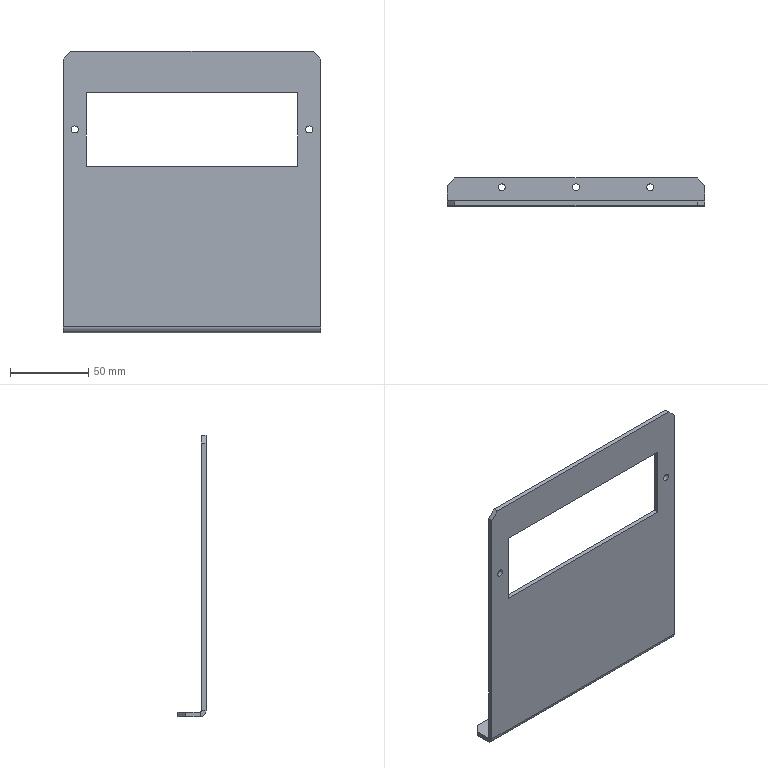Part | NX | 1 solid | 27 faces | box 165 x 18 x 180 mm | volume 76623 mm3 | plane 20 | cylinder 7 | commonest cylinder face diameters 4.5 x5 1.5 x1 7.5 x1
STEP:
#1=CARTESIAN_POINT('',(82.5,0.,3.75));
#2=VERTEX_POINT('',#1);
#3=CARTESIAN_POINT('',(82.5,3.,3.75));
#4=VERTEX_POINT('',#3);
#5=CARTESIAN_POINT('',(82.5,0.,3.75));
#6=DIRECTION('',(0.,1.,0.));
#7=VECTOR('',#6,1000.);
#8=LINE('',#5,#7);
#9=EDGE_CURVE('',#2,#4,#8,.T.);
#10=ORIENTED_EDGE('',*,*,#9,.F.);
#11=CARTESIAN_POINT('',(82.5,3.75,0.));
#12=VERTEX_POINT('',#11);
#13=CARTESIAN_POINT('',(82.5,3.75,3.75));
#14=DIRECTION('',(1.,0.,0.));
#15=DIRECTION('',(0.,0.,-1.));
#16=AXIS2_PLACEMENT_3D('',#13,#14,#15);
#17=CIRCLE('',#16,3.75);
#18=EDGE_CURVE('',#12,#2,#17,.F.);
#19=ORIENTED_EDGE('',*,*,#18,.F.);
#20=CARTESIAN_POINT('',(82.5,3.75,3.));
#21=VERTEX_POINT('',#20);
#22=CARTESIAN_POINT('',(82.5,3.75,3.));
#23=DIRECTION('',(0.,0.,-1.));
#24=VECTOR('',#23,1000.);
#25=LINE('',#22,#24);
#26=EDGE_CURVE('',#21,#12,#25,.T.);
#27=ORIENTED_EDGE('',*,*,#26,.F.);
#28=CARTESIAN_POINT('',(82.5,3.75,3.75));
#29=DIRECTION('',(1.,0.,0.));
#30=DIRECTION('',(0.,0.,-1.));
#31=AXIS2_PLACEMENT_3D('',#28,#29,#30);
#32=CIRCLE('',#31,0.75);
#33=EDGE_CURVE('',#21,#4,#32,.F.);
#34=ORIENTED_EDGE('',*,*,#33,.T.);
#35=EDGE_LOOP('',(#10,#19,#27,#34));
#36=FACE_BOUND('',#35,.T.);
#37=CARTESIAN_POINT('',(82.5,0.,3.75));
#38=DIRECTION('',(1.,0.,0.));
#39=DIRECTION('',(0.,0.,-1.));
#40=AXIS2_PLACEMENT_3D('',#37,#38,#39);
#41=PLANE('',#40);
#42=ADVANCED_FACE('',(#36),#41,.T.);
#43=CARTESIAN_POINT('',(82.5,3.,175.));
#44=VERTEX_POINT('',#43);
#45=CARTESIAN_POINT('',(82.5,3.,0.));
#46=DIRECTION('',(0.,0.,1.));
#47=VECTOR('',#46,1000.);
#48=LINE('',#45,#47);
#49=EDGE_CURVE('',#4,#44,#48,.T.);
#50=ORIENTED_EDGE('',*,*,#49,.T.);
#51=CARTESIAN_POINT('',(82.5,0.,175.));
#52=VERTEX_POINT('',#51);
#53=CARTESIAN_POINT('',(82.5,3.75,175.));
#54=DIRECTION('',(0.,-1.,0.));
#55=VECTOR('',#54,1000.);
#56=LINE('',#53,#55);
#57=EDGE_CURVE('',#44,#52,#56,.T.);
#58=ORIENTED_EDGE('',*,*,#57,.T.);
#59=CARTESIAN_POINT('',(82.5,0.,0.));
#60=DIRECTION('',(0.,0.,1.));
#61=VECTOR('',#60,1000.);
#62=LINE('',#59,#61);
#63=EDGE_CURVE('',#2,#52,#62,.T.);
#64=ORIENTED_EDGE('',*,*,#63,.F.);
#65=ORIENTED_EDGE('',*,*,#9,.T.);
#66=EDGE_LOOP('',(#50,#58,#64,#65));
#67=FACE_BOUND('',#66,.T.);
#68=CARTESIAN_POINT('',(82.5,3.75,3.));
#69=DIRECTION('',(1.,0.,0.));
#70=DIRECTION('',(0.,0.,-1.));
#71=AXIS2_PLACEMENT_3D('',#68,#69,#70);
#72=PLANE('',#71);
#73=ADVANCED_FACE('',(#67),#72,.T.);
#74=CARTESIAN_POINT('',(-82.5,3.75,0.));
#75=VERTEX_POINT('',#74);
#76=CARTESIAN_POINT('',(-82.5,3.75,3.));
#77=VERTEX_POINT('',#76);
#78=CARTESIAN_POINT('',(-82.5,3.75,0.));
#79=DIRECTION('',(0.,0.,1.));
#80=VECTOR('',#79,1000.);
#81=LINE('',#78,#80);
#82=EDGE_CURVE('',#75,#77,#81,.T.);
#83=ORIENTED_EDGE('',*,*,#82,.F.);
#84=CARTESIAN_POINT('',(-82.5,0.,3.75));
#85=VERTEX_POINT('',#84);
#86=CARTESIAN_POINT('',(-82.5,3.75,3.75));
#87=DIRECTION('',(1.,0.,0.));
#88=DIRECTION('',(0.,0.,-1.));
#89=AXIS2_PLACEMENT_3D('',#86,#87,#88);
#90=CIRCLE('',#89,3.75);
#91=EDGE_CURVE('',#75,#85,#90,.F.);
#92=ORIENTED_EDGE('',*,*,#91,.T.);
#93=CARTESIAN_POINT('',(-82.5,3.,3.75));
#94=VERTEX_POINT('',#93);
#95=CARTESIAN_POINT('',(-82.5,3.,3.75));
#96=DIRECTION('',(0.,-1.,0.));
#97=VECTOR('',#96,1000.);
#98=LINE('',#95,#97);
#99=EDGE_CURVE('',#94,#85,#98,.T.);
#100=ORIENTED_EDGE('',*,*,#99,.F.);
#101=CARTESIAN_POINT('',(-82.5,3.75,3.75));
#102=DIRECTION('',(1.,0.,0.));
#103=DIRECTION('',(0.,0.,-1.));
#104=AXIS2_PLACEMENT_3D('',#101,#102,#103);
#105=CIRCLE('',#104,0.75);
#106=EDGE_CURVE('',#77,#94,#105,.F.);
#107=ORIENTED_EDGE('',*,*,#106,.F.);
#108=EDGE_LOOP('',(#83,#92,#100,#107));
#109=FACE_BOUND('',#108,.T.);
#110=CARTESIAN_POINT('',(-82.5,3.75,0.));
#111=DIRECTION('',(-1.,0.,0.));
#112=DIRECTION('',(0.,0.,1.));
#113=AXIS2_PLACEMENT_3D('',#110,#111,#112);
#114=PLANE('',#113);
#115=ADVANCED_FACE('',(#109),#114,.T.);
#116=CARTESIAN_POINT('',(-82.5,13.,3.));
#117=VERTEX_POINT('',#116);
#118=CARTESIAN_POINT('',(-82.5,18.,3.));
#119=DIRECTION('',(0.,-1.,0.));
#120=VECTOR('',#119,1000.);
#121=LINE('',#118,#120);
#122=EDGE_CURVE('',#117,#77,#121,.T.);
#123=ORIENTED_EDGE('',*,*,#122,.F.);
#124=CARTESIAN_POINT('',(-82.5,13.,0.));
#125=VERTEX_POINT('',#124);
#126=CARTESIAN_POINT('',(-82.5,13.,3.75));
#127=DIRECTION('',(0.,0.,-1.));
#128=VECTOR('',#127,1000.);
#129=LINE('',#126,#128);
#130=EDGE_CURVE('',#117,#125,#129,.T.);
#131=ORIENTED_EDGE('',*,*,#130,.T.);
#132=CARTESIAN_POINT('',(-82.5,18.,0.));
#133=DIRECTION('',(0.,-1.,0.));
#134=VECTOR('',#133,1000.);
#135=LINE('',#132,#134);
#136=EDGE_CURVE('',#125,#75,#135,.T.);
#137=ORIENTED_EDGE('',*,*,#136,.T.);
#138=ORIENTED_EDGE('',*,*,#82,.T.);
#139=EDGE_LOOP('',(#123,#131,#137,#138));
#140=FACE_BOUND('',#139,.T.);
#141=CARTESIAN_POINT('',(-82.5,3.,3.75));
#142=DIRECTION('',(-1.,0.,0.));
#143=DIRECTION('',(0.,0.,1.));
#144=AXIS2_PLACEMENT_3D('',#141,#142,#143);
#145=PLANE('',#144);
#146=ADVANCED_FACE('',(#140),#145,.T.);
#147=CARTESIAN_POINT('',(-67.5,3.,106.5));
#148=VERTEX_POINT('',#147);
#149=CARTESIAN_POINT('',(67.5,3.,106.5));
#150=VERTEX_POINT('',#149);
#151=CARTESIAN_POINT('',(82.5,3.,106.5));
#152=DIRECTION('',(1.,0.,0.));
#153=VECTOR('',#152,1000.);
#154=LINE('',#151,#153);
#155=EDGE_CURVE('',#148,#150,#154,.T.);
#156=ORIENTED_EDGE('',*,*,#155,.T.);
#157=CARTESIAN_POINT('',(67.5,3.,153.5));
#158=VERTEX_POINT('',#157);
#159=CARTESIAN_POINT('',(67.5,3.,0.));
#160=DIRECTION('',(0.,0.,1.));
#161=VECTOR('',#160,1000.);
#162=LINE('',#159,#161);
#163=EDGE_CURVE('',#150,#158,#162,.T.);
#164=ORIENTED_EDGE('',*,*,#163,.T.);
#165=CARTESIAN_POINT('',(-67.5,3.,153.5));
#166=VERTEX_POINT('',#165);
#167=CARTESIAN_POINT('',(82.5,3.,153.5));
#168=DIRECTION('',(-1.,0.,0.));
#169=VECTOR('',#168,1000.);
#170=LINE('',#167,#169);
#171=EDGE_CURVE('',#158,#166,#170,.T.);
#172=ORIENTED_EDGE('',*,*,#171,.T.);
#173=CARTESIAN_POINT('',(-67.5,3.,0.));
#174=DIRECTION('',(0.,0.,-1.));
#175=VECTOR('',#174,1000.);
#176=LINE('',#173,#175);
#177=EDGE_CURVE('',#166,#148,#176,.T.);
#178=ORIENTED_EDGE('',*,*,#177,.T.);
#179=EDGE_LOOP('',(#156,#164,#172,#178));
#180=FACE_BOUND('',#179,.T.);
#181=CARTESIAN_POINT('',(75.,3.,127.75));
#182=VERTEX_POINT('',#181);
#183=CARTESIAN_POINT('',(75.,3.,130.));
#184=DIRECTION('',(0.,-1.,0.));
#185=DIRECTION('',(0.,0.,-1.));
#186=AXIS2_PLACEMENT_3D('',#183,#184,#185);
#187=CIRCLE('',#186,2.25);
#188=EDGE_CURVE('',#182,#182,#187,.T.);
#189=ORIENTED_EDGE('',*,*,#188,.T.);
#190=EDGE_LOOP('',(#189));
#191=FACE_BOUND('',#190,.T.);
#192=CARTESIAN_POINT('',(-75.,3.,127.75));
#193=VERTEX_POINT('',#192);
#194=CARTESIAN_POINT('',(-75.,3.,130.));
#195=DIRECTION('',(0.,-1.,0.));
#196=DIRECTION('',(0.,0.,-1.));
#197=AXIS2_PLACEMENT_3D('',#194,#195,#196);
#198=CIRCLE('',#197,2.25);
#199=EDGE_CURVE('',#193,#193,#198,.T.);
#200=ORIENTED_EDGE('',*,*,#199,.T.);
#201=EDGE_LOOP('',(#200));
#202=FACE_BOUND('',#201,.T.);
#203=CARTESIAN_POINT('',(77.5,3.,180.));
#204=VERTEX_POINT('',#203);
#205=CARTESIAN_POINT('',(-77.5,3.,180.));
#206=VERTEX_POINT('',#205);
#207=CARTESIAN_POINT('',(82.5,3.,180.));
#208=DIRECTION('',(-1.,0.,0.));
#209=VECTOR('',#208,1000.);
#210=LINE('',#207,#209);
#211=EDGE_CURVE('',#204,#206,#210,.T.);
#212=ORIENTED_EDGE('',*,*,#211,.F.);
#213=CARTESIAN_POINT('',(77.5,3.,180.));
#214=DIRECTION('',(-0.7071,0.,0.7071));
#215=VECTOR('',#214,1000.);
#216=LINE('',#213,#215);
#217=EDGE_CURVE('',#204,#44,#216,.F.);
#218=ORIENTED_EDGE('',*,*,#217,.T.);
#219=ORIENTED_EDGE('',*,*,#49,.F.);
#220=CARTESIAN_POINT('',(82.5,3.,3.75));
#221=DIRECTION('',(-1.,0.,0.));
#222=VECTOR('',#221,1000.);
#223=LINE('',#220,#222);
#224=EDGE_CURVE('',#4,#94,#223,.T.);
#225=ORIENTED_EDGE('',*,*,#224,.T.);
#226=CARTESIAN_POINT('',(-82.5,3.,175.));
#227=VERTEX_POINT('',#226);
#228=CARTESIAN_POINT('',(-82.5,3.,0.));
#229=DIRECTION('',(0.,0.,1.));
#230=VECTOR('',#229,1000.);
#231=LINE('',#228,#230);
#232=EDGE_CURVE('',#94,#227,#231,.T.);
#233=ORIENTED_EDGE('',*,*,#232,.T.);
#234=CARTESIAN_POINT('',(-82.5,3.,175.));
#235=DIRECTION('',(0.7071,0.,0.7071));
#236=VECTOR('',#235,1000.);
#237=LINE('',#234,#236);
#238=EDGE_CURVE('',#227,#206,#237,.T.);
#239=ORIENTED_EDGE('',*,*,#238,.T.);
#240=EDGE_LOOP('',(#212,#218,#219,#225,#233,#239));
#241=FACE_BOUND('',#240,.T.);
#242=CARTESIAN_POINT('',(82.5,3.,0.));
#243=DIRECTION('',(0.,-1.,0.));
#244=DIRECTION('',(0.,0.,-1.));
#245=AXIS2_PLACEMENT_3D('',#242,#243,#244);
#246=PLANE('',#245);
#247=ADVANCED_FACE('',(#180,#191,#202,#241),#246,.F.);
#248=CARTESIAN_POINT('',(77.5,0.,180.));
#249=VERTEX_POINT('',#248);
#250=CARTESIAN_POINT('',(-77.5,0.,180.));
#251=VERTEX_POINT('',#250);
#252=CARTESIAN_POINT('',(82.5,0.,180.));
#253=DIRECTION('',(-1.,0.,0.));
#254=VECTOR('',#253,1000.);
#255=LINE('',#252,#254);
#256=EDGE_CURVE('',#249,#251,#255,.T.);
#257=ORIENTED_EDGE('',*,*,#256,.F.);
#258=CARTESIAN_POINT('',(77.5,0.,180.));
#259=DIRECTION('',(0.,1.,0.));
#260=VECTOR('',#259,1000.);
#261=LINE('',#258,#260);
#262=EDGE_CURVE('',#249,#204,#261,.T.);
#263=ORIENTED_EDGE('',*,*,#262,.T.);
#264=ORIENTED_EDGE('',*,*,#211,.T.);
#265=CARTESIAN_POINT('',(-77.5,0.,180.));
#266=DIRECTION('',(0.,-1.,0.));
#267=VECTOR('',#266,1000.);
#268=LINE('',#265,#267);
#269=EDGE_CURVE('',#206,#251,#268,.T.);
#270=ORIENTED_EDGE('',*,*,#269,.T.);
#271=EDGE_LOOP('',(#257,#263,#264,#270));
#272=FACE_BOUND('',#271,.T.);
#273=CARTESIAN_POINT('',(82.5,0.,180.));
#274=DIRECTION('',(0.,0.,1.));
#275=DIRECTION('',(1.,0.,0.));
#276=AXIS2_PLACEMENT_3D('',#273,#274,#275);
#277=PLANE('',#276);
#278=ADVANCED_FACE('',(#272),#277,.T.);
#279=CARTESIAN_POINT('',(67.5,0.,106.5));
#280=VERTEX_POINT('',#279);
#281=CARTESIAN_POINT('',(67.5,0.,153.5));
#282=VERTEX_POINT('',#281);
#283=CARTESIAN_POINT('',(67.5,0.,106.5));
#284=DIRECTION('',(0.,0.,1.));
#285=VECTOR('',#284,1000.);
#286=LINE('',#283,#285);
#287=EDGE_CURVE('',#280,#282,#286,.T.);
#288=ORIENTED_EDGE('',*,*,#287,.F.);
#289=CARTESIAN_POINT('',(-67.5,0.,106.5));
#290=VERTEX_POINT('',#289);
#291=CARTESIAN_POINT('',(-67.5,0.,106.5));
#292=DIRECTION('',(1.,0.,0.));
#293=VECTOR('',#292,1000.);
#294=LINE('',#291,#293);
#295=EDGE_CURVE('',#290,#280,#294,.T.);
#296=ORIENTED_EDGE('',*,*,#295,.F.);
#297=CARTESIAN_POINT('',(-67.5,0.,153.5));
#298=VERTEX_POINT('',#297);
#299=CARTESIAN_POINT('',(-67.5,0.,106.5));
#300=DIRECTION('',(0.,0.,-1.));
#301=VECTOR('',#300,1000.);
#302=LINE('',#299,#301);
#303=EDGE_CURVE('',#298,#290,#302,.T.);
#304=ORIENTED_EDGE('',*,*,#303,.F.);
#305=CARTESIAN_POINT('',(-67.5,0.,153.5));
#306=DIRECTION('',(-1.,0.,0.));
#307=VECTOR('',#306,1000.);
#308=LINE('',#305,#307);
#309=EDGE_CURVE('',#282,#298,#308,.T.);
#310=ORIENTED_EDGE('',*,*,#309,.F.);
#311=EDGE_LOOP('',(#288,#296,#304,#310));
#312=FACE_BOUND('',#311,.T.);
#313=CARTESIAN_POINT('',(75.,0.,127.75));
#314=VERTEX_POINT('',#313);
#315=CARTESIAN_POINT('',(75.,0.,130.));
#316=DIRECTION('',(0.,-1.,0.));
#317=DIRECTION('',(0.,0.,-1.));
#318=AXIS2_PLACEMENT_3D('',#315,#316,#317);
#319=CIRCLE('',#318,2.25);
#320=EDGE_CURVE('',#314,#314,#319,.T.);
#321=ORIENTED_EDGE('',*,*,#320,.F.);
#322=EDGE_LOOP('',(#321));
#323=FACE_BOUND('',#322,.T.);
#324=CARTESIAN_POINT('',(-75.,0.,127.75));
#325=VERTEX_POINT('',#324);
#326=CARTESIAN_POINT('',(-75.,0.,130.));
#327=DIRECTION('',(0.,-1.,0.));
#328=DIRECTION('',(0.,0.,-1.));
#329=AXIS2_PLACEMENT_3D('',#326,#327,#328);
#330=CIRCLE('',#329,2.25);
#331=EDGE_CURVE('',#325,#325,#330,.T.);
#332=ORIENTED_EDGE('',*,*,#331,.F.);
#333=EDGE_LOOP('',(#332));
#334=FACE_BOUND('',#333,.T.);
#335=ORIENTED_EDGE('',*,*,#63,.T.);
#336=CARTESIAN_POINT('',(170.,0.,87.5));
#337=DIRECTION('',(0.7071,0.,-0.7071));
#338=VECTOR('',#337,1000.);
#339=LINE('',#336,#338);
#340=EDGE_CURVE('',#52,#249,#339,.F.);
#341=ORIENTED_EDGE('',*,*,#340,.T.);
#342=ORIENTED_EDGE('',*,*,#256,.T.);
#343=CARTESIAN_POINT('',(-82.5,0.,175.));
#344=VERTEX_POINT('',#343);
#345=CARTESIAN_POINT('',(-87.5,0.,170.));
#346=DIRECTION('',(-0.7071,0.,-0.7071));
#347=VECTOR('',#346,1000.);
#348=LINE('',#345,#347);
#349=EDGE_CURVE('',#251,#344,#348,.T.);
#350=ORIENTED_EDGE('',*,*,#349,.T.);
#351=CARTESIAN_POINT('',(-82.5,0.,0.));
#352=DIRECTION('',(0.,0.,1.));
#353=VECTOR('',#352,1000.);
#354=LINE('',#351,#353);
#355=EDGE_CURVE('',#85,#344,#354,.T.);
#356=ORIENTED_EDGE('',*,*,#355,.F.);
#357=CARTESIAN_POINT('',(82.5,0.,3.75));
#358=DIRECTION('',(-1.,0.,0.));
#359=VECTOR('',#358,1000.);
#360=LINE('',#357,#359);
#361=EDGE_CURVE('',#2,#85,#360,.T.);
#362=ORIENTED_EDGE('',*,*,#361,.F.);
#363=EDGE_LOOP('',(#335,#341,#342,#350,#356,#362));
#364=FACE_BOUND('',#363,.T.);
#365=CARTESIAN_POINT('',(82.5,0.,0.));
#366=DIRECTION('',(0.,-1.,0.));
#367=DIRECTION('',(0.,0.,-1.));
#368=AXIS2_PLACEMENT_3D('',#365,#366,#367);
#369=PLANE('',#368);
#370=ADVANCED_FACE('',(#312,#323,#334,#364),#369,.T.);
#371=ORIENTED_EDGE('',*,*,#91,.F.);
#372=CARTESIAN_POINT('',(82.5,3.75,0.));
#373=DIRECTION('',(-1.,0.,0.));
#374=VECTOR('',#373,1000.);
#375=LINE('',#372,#374);
#376=EDGE_CURVE('',#12,#75,#375,.T.);
#377=ORIENTED_EDGE('',*,*,#376,.F.);
#378=ORIENTED_EDGE('',*,*,#18,.T.);
#379=ORIENTED_EDGE('',*,*,#361,.T.);
#380=EDGE_LOOP('',(#371,#377,#378,#379));
#381=FACE_BOUND('',#380,.T.);
#382=CARTESIAN_POINT('',(82.5,3.75,3.75));
#383=DIRECTION('',(-1.,0.,0.));
#384=DIRECTION('',(0.,0.,1.));
#385=AXIS2_PLACEMENT_3D('',#382,#383,#384);
#386=CYLINDRICAL_SURFACE('',#385,3.75);
#387=ADVANCED_FACE('',(#381),#386,.T.);
#388=CARTESIAN_POINT('',(-45.25,12.,0.));
#389=VERTEX_POINT('',#388);
#390=CARTESIAN_POINT('',(-47.5,12.,0.));
#391=DIRECTION('',(0.,0.,1.));
#392=DIRECTION('',(1.,0.,0.));
#393=AXIS2_PLACEMENT_3D('',#390,#391,#392);
#394=CIRCLE('',#393,2.25);
#395=EDGE_CURVE('',#389,#389,#394,.T.);
#396=ORIENTED_EDGE('',*,*,#395,.T.);
#397=EDGE_LOOP('',(#396));
#398=FACE_BOUND('',#397,.T.);
#399=CARTESIAN_POINT('',(49.75,12.,0.));
#400=VERTEX_POINT('',#399);
#401=CARTESIAN_POINT('',(47.5,12.,0.));
#402=DIRECTION('',(0.,0.,1.));
#403=DIRECTION('',(1.,0.,0.));
#404=AXIS2_PLACEMENT_3D('',#401,#402,#403);
#405=CIRCLE('',#404,2.25);
#406=EDGE_CURVE('',#400,#400,#405,.T.);
#407=ORIENTED_EDGE('',*,*,#406,.T.);
#408=EDGE_LOOP('',(#407));
#409=FACE_BOUND('',#408,.T.);
#410=CARTESIAN_POINT('',(2.25,12.,0.));
#411=VERTEX_POINT('',#410);
#412=CARTESIAN_POINT('',(0.,12.,0.));
#413=DIRECTION('',(0.,0.,1.));
#414=DIRECTION('',(1.,0.,0.));
#415=AXIS2_PLACEMENT_3D('',#412,#413,#414);
#416=CIRCLE('',#415,2.25);
#417=EDGE_CURVE('',#411,#411,#416,.T.);
#418=ORIENTED_EDGE('',*,*,#417,.T.);
#419=EDGE_LOOP('',(#418));
#420=FACE_BOUND('',#419,.T.);
#421=CARTESIAN_POINT('',(77.5,18.,0.));
#422=VERTEX_POINT('',#421);
#423=CARTESIAN_POINT('',(-77.5,18.,0.));
#424=VERTEX_POINT('',#423);
#425=CARTESIAN_POINT('',(82.5,18.,0.));
#426=DIRECTION('',(-1.,0.,0.));
#427=VECTOR('',#426,1000.);
#428=LINE('',#425,#427);
#429=EDGE_CURVE('',#422,#424,#428,.T.);
#430=ORIENTED_EDGE('',*,*,#429,.F.);
#431=CARTESIAN_POINT('',(82.5,13.,0.));
#432=VERTEX_POINT('',#431);
#433=CARTESIAN_POINT('',(80.,15.5,0.));
#434=DIRECTION('',(-0.7071,0.7071,0.));
#435=VECTOR('',#434,1000.);
#436=LINE('',#433,#435);
#437=EDGE_CURVE('',#422,#432,#436,.F.);
#438=ORIENTED_EDGE('',*,*,#437,.T.);
#439=CARTESIAN_POINT('',(82.5,18.,0.));
#440=DIRECTION('',(0.,-1.,0.));
#441=VECTOR('',#440,1000.);
#442=LINE('',#439,#441);
#443=EDGE_CURVE('',#432,#12,#442,.T.);
#444=ORIENTED_EDGE('',*,*,#443,.T.);
#445=ORIENTED_EDGE('',*,*,#376,.T.);
#446=ORIENTED_EDGE('',*,*,#136,.F.);
#447=CARTESIAN_POINT('',(2.5,98.,0.));
#448=DIRECTION('',(-0.7071,-0.7071,0.));
#449=VECTOR('',#448,1000.);
#450=LINE('',#447,#449);
#451=EDGE_CURVE('',#125,#424,#450,.F.);
#452=ORIENTED_EDGE('',*,*,#451,.T.);
#453=EDGE_LOOP('',(#430,#438,#444,#445,#446,#452));
#454=FACE_BOUND('',#453,.T.);
#455=CARTESIAN_POINT('',(82.5,18.,0.));
#456=DIRECTION('',(0.,0.,-1.));
#457=DIRECTION('',(0.,1.,0.));
#458=AXIS2_PLACEMENT_3D('',#455,#456,#457);
#459=PLANE('',#458);
#460=ADVANCED_FACE('',(#398,#409,#420,#454),#459,.T.);
#461=CARTESIAN_POINT('',(77.5,18.,3.));
#462=VERTEX_POINT('',#461);
#463=CARTESIAN_POINT('',(-77.5,18.,3.));
#464=VERTEX_POINT('',#463);
#465=CARTESIAN_POINT('',(82.5,18.,3.));
#466=DIRECTION('',(-1.,0.,0.));
#467=VECTOR('',#466,1000.);
#468=LINE('',#465,#467);
#469=EDGE_CURVE('',#462,#464,#468,.T.);
#470=ORIENTED_EDGE('',*,*,#469,.F.);
#471=CARTESIAN_POINT('',(77.5,18.,3.));
#472=DIRECTION('',(0.,0.,-1.));
#473=VECTOR('',#472,1000.);
#474=LINE('',#471,#473);
#475=EDGE_CURVE('',#462,#422,#474,.T.);
#476=ORIENTED_EDGE('',*,*,#475,.T.);
#477=ORIENTED_EDGE('',*,*,#429,.T.);
#478=CARTESIAN_POINT('',(-77.5,18.,3.));
#479=DIRECTION('',(0.,0.,1.));
#480=VECTOR('',#479,1000.);
#481=LINE('',#478,#480);
#482=EDGE_CURVE('',#424,#464,#481,.T.);
#483=ORIENTED_EDGE('',*,*,#482,.T.);
#484=EDGE_LOOP('',(#470,#476,#477,#483));
#485=FACE_BOUND('',#484,.T.);
#486=CARTESIAN_POINT('',(82.5,18.,3.));
#487=DIRECTION('',(0.,1.,0.));
#488=DIRECTION('',(0.,0.,1.));
#489=AXIS2_PLACEMENT_3D('',#486,#487,#488);
#490=PLANE('',#489);
#491=ADVANCED_FACE('',(#485),#490,.T.);
#492=CARTESIAN_POINT('',(-45.25,12.,3.));
#493=VERTEX_POINT('',#492);
#494=CARTESIAN_POINT('',(-47.5,12.,3.));
#495=DIRECTION('',(0.,0.,1.));
#496=DIRECTION('',(1.,0.,0.));
#497=AXIS2_PLACEMENT_3D('',#494,#495,#496);
#498=CIRCLE('',#497,2.25);
#499=EDGE_CURVE('',#493,#493,#498,.T.);
#500=ORIENTED_EDGE('',*,*,#499,.F.);
#501=EDGE_LOOP('',(#500));
#502=FACE_BOUND('',#501,.T.);
#503=CARTESIAN_POINT('',(49.75,12.,3.));
#504=VERTEX_POINT('',#503);
#505=CARTESIAN_POINT('',(47.5,12.,3.));
#506=DIRECTION('',(0.,0.,1.));
#507=DIRECTION('',(1.,0.,0.));
#508=AXIS2_PLACEMENT_3D('',#505,#506,#507);
#509=CIRCLE('',#508,2.25);
#510=EDGE_CURVE('',#504,#504,#509,.T.);
#511=ORIENTED_EDGE('',*,*,#510,.F.);
#512=EDGE_LOOP('',(#511));
#513=FACE_BOUND('',#512,.T.);
#514=CARTESIAN_POINT('',(2.25,12.,3.));
#515=VERTEX_POINT('',#514);
#516=CARTESIAN_POINT('',(0.,12.,3.));
#517=DIRECTION('',(0.,0.,1.));
#518=DIRECTION('',(1.,0.,0.));
#519=AXIS2_PLACEMENT_3D('',#516,#517,#518);
#520=CIRCLE('',#519,2.25);
#521=EDGE_CURVE('',#515,#515,#520,.T.);
#522=ORIENTED_EDGE('',*,*,#521,.F.);
#523=EDGE_LOOP('',(#522));
#524=FACE_BOUND('',#523,.T.);
#525=CARTESIAN_POINT('',(82.5,13.,3.));
#526=VERTEX_POINT('',#525);
#527=CARTESIAN_POINT('',(82.5,18.,3.));
#528=DIRECTION('',(0.,-1.,0.));
#529=VECTOR('',#528,1000.);
#530=LINE('',#527,#529);
#531=EDGE_CURVE('',#526,#21,#530,.T.);
#532=ORIENTED_EDGE('',*,*,#531,.F.);
#533=CARTESIAN_POINT('',(77.5,18.,3.));
#534=DIRECTION('',(0.7071,-0.7071,0.));
#535=VECTOR('',#534,1000.);
#536=LINE('',#533,#535);
#537=EDGE_CURVE('',#526,#462,#536,.F.);
#538=ORIENTED_EDGE('',*,*,#537,.T.);
#539=ORIENTED_EDGE('',*,*,#469,.T.);
#540=CARTESIAN_POINT('',(-82.5,13.,3.));
#541=DIRECTION('',(0.7071,0.7071,0.));
#542=VECTOR('',#541,1000.);
#543=LINE('',#540,#542);
#544=EDGE_CURVE('',#464,#117,#543,.F.);
#545=ORIENTED_EDGE('',*,*,#544,.T.);
#546=ORIENTED_EDGE('',*,*,#122,.T.);
#547=CARTESIAN_POINT('',(82.5,3.75,3.));
#548=DIRECTION('',(-1.,0.,0.));
#549=VECTOR('',#548,1000.);
#550=LINE('',#547,#549);
#551=EDGE_CURVE('',#21,#77,#550,.T.);
#552=ORIENTED_EDGE('',*,*,#551,.F.);
#553=EDGE_LOOP('',(#532,#538,#539,#545,#546,#552));
#554=FACE_BOUND('',#553,.T.);
#555=CARTESIAN_POINT('',(82.5,18.,3.));
#556=DIRECTION('',(0.,0.,-1.));
#557=DIRECTION('',(0.,1.,0.));
#558=AXIS2_PLACEMENT_3D('',#555,#556,#557);
#559=PLANE('',#558);
#560=ADVANCED_FACE('',(#502,#513,#524,#554),#559,.F.);
#561=ORIENTED_EDGE('',*,*,#106,.T.);
#562=ORIENTED_EDGE('',*,*,#224,.F.);
#563=ORIENTED_EDGE('',*,*,#33,.F.);
#564=ORIENTED_EDGE('',*,*,#551,.T.);
#565=EDGE_LOOP('',(#561,#562,#563,#564));
#566=FACE_BOUND('',#565,.T.);
#567=CARTESIAN_POINT('',(82.5,3.75,3.75));
#568=DIRECTION('',(-1.,0.,0.));
#569=DIRECTION('',(0.,0.,1.));
#570=AXIS2_PLACEMENT_3D('',#567,#568,#569);
#571=CYLINDRICAL_SURFACE('',#570,0.75);
#572=ADVANCED_FACE('',(#566),#571,.F.);
#573=ORIENTED_EDGE('',*,*,#443,.F.);
#574=CARTESIAN_POINT('',(82.5,13.,3.75));
#575=DIRECTION('',(0.,0.,1.));
#576=VECTOR('',#575,1000.);
#577=LINE('',#574,#576);
#578=EDGE_CURVE('',#432,#526,#577,.T.);
#579=ORIENTED_EDGE('',*,*,#578,.T.);
#580=ORIENTED_EDGE('',*,*,#531,.T.);
#581=ORIENTED_EDGE('',*,*,#26,.T.);
#582=EDGE_LOOP('',(#573,#579,#580,#581));
#583=FACE_BOUND('',#582,.T.);
#584=CARTESIAN_POINT('',(82.5,3.75,3.75));
#585=DIRECTION('',(1.,0.,0.));
#586=DIRECTION('',(0.,0.,-1.));
#587=AXIS2_PLACEMENT_3D('',#584,#585,#586);
#588=PLANE('',#587);
#589=ADVANCED_FACE('',(#583),#588,.T.);
#590=ORIENTED_EDGE('',*,*,#355,.T.);
#591=CARTESIAN_POINT('',(-82.5,3.,175.));
#592=DIRECTION('',(0.,1.,0.));
#593=VECTOR('',#592,1000.);
#594=LINE('',#591,#593);
#595=EDGE_CURVE('',#344,#227,#594,.T.);
#596=ORIENTED_EDGE('',*,*,#595,.T.);
#597=ORIENTED_EDGE('',*,*,#232,.F.);
#598=ORIENTED_EDGE('',*,*,#99,.T.);
#599=EDGE_LOOP('',(#590,#596,#597,#598));
#600=FACE_BOUND('',#599,.T.);
#601=CARTESIAN_POINT('',(-82.5,3.75,3.75));
#602=DIRECTION('',(1.,0.,0.));
#603=DIRECTION('',(0.,0.,-1.));
#604=AXIS2_PLACEMENT_3D('',#601,#602,#603);
#605=PLANE('',#604);
#606=ADVANCED_FACE('',(#600),#605,.F.);
#607=ORIENTED_EDGE('',*,*,#331,.T.);
#608=EDGE_LOOP('',(#607));
#609=FACE_BOUND('',#608,.T.);
#610=ORIENTED_EDGE('',*,*,#199,.F.);
#611=EDGE_LOOP('',(#610));
#612=FACE_BOUND('',#611,.T.);
#613=CARTESIAN_POINT('',(-75.,0.,130.));
#614=DIRECTION('',(0.,-1.,0.));
#615=DIRECTION('',(0.,0.,-1.));
#616=AXIS2_PLACEMENT_3D('',#613,#614,#615);
#617=CYLINDRICAL_SURFACE('',#616,2.25);
#618=ADVANCED_FACE('',(#609,#612),#617,.F.);
#619=ORIENTED_EDGE('',*,*,#320,.T.);
#620=EDGE_LOOP('',(#619));
#621=FACE_BOUND('',#620,.T.);
#622=ORIENTED_EDGE('',*,*,#188,.F.);
#623=EDGE_LOOP('',(#622));
#624=FACE_BOUND('',#623,.T.);
#625=CARTESIAN_POINT('',(75.,0.,130.));
#626=DIRECTION('',(0.,-1.,0.));
#627=DIRECTION('',(0.,0.,-1.));
#628=AXIS2_PLACEMENT_3D('',#625,#626,#627);
#629=CYLINDRICAL_SURFACE('',#628,2.25);
#630=ADVANCED_FACE('',(#621,#624),#629,.F.);
#631=ORIENTED_EDGE('',*,*,#537,.F.);
#632=ORIENTED_EDGE('',*,*,#578,.F.);
#633=ORIENTED_EDGE('',*,*,#437,.F.);
#634=ORIENTED_EDGE('',*,*,#475,.F.);
#635=EDGE_LOOP('',(#631,#632,#633,#634));
#636=FACE_BOUND('',#635,.T.);
#637=CARTESIAN_POINT('',(77.5,18.,3.));
#638=DIRECTION('',(-0.7071,-0.7071,0.));
#639=DIRECTION('',(0.,0.,-1.));
#640=AXIS2_PLACEMENT_3D('',#637,#638,#639);
#641=PLANE('',#640);
#642=ADVANCED_FACE('',(#636),#641,.F.);
#643=ORIENTED_EDGE('',*,*,#544,.F.);
#644=ORIENTED_EDGE('',*,*,#482,.F.);
#645=ORIENTED_EDGE('',*,*,#451,.F.);
#646=ORIENTED_EDGE('',*,*,#130,.F.);
#647=EDGE_LOOP('',(#643,#644,#645,#646));
#648=FACE_BOUND('',#647,.T.);
#649=CARTESIAN_POINT('',(-82.5,13.,3.75));
#650=DIRECTION('',(0.7071,-0.7071,0.));
#651=DIRECTION('',(0.,0.,-1.));
#652=AXIS2_PLACEMENT_3D('',#649,#650,#651);
#653=PLANE('',#652);
#654=ADVANCED_FACE('',(#648),#653,.F.);
#655=ORIENTED_EDGE('',*,*,#340,.F.);
#656=ORIENTED_EDGE('',*,*,#57,.F.);
#657=ORIENTED_EDGE('',*,*,#217,.F.);
#658=ORIENTED_EDGE('',*,*,#262,.F.);
#659=EDGE_LOOP('',(#655,#656,#657,#658));
#660=FACE_BOUND('',#659,.T.);
#661=CARTESIAN_POINT('',(77.5,0.,180.));
#662=DIRECTION('',(-0.7071,0.,-0.7071));
#663=DIRECTION('',(0.,1.,0.));
#664=AXIS2_PLACEMENT_3D('',#661,#662,#663);
#665=PLANE('',#664);
#666=ADVANCED_FACE('',(#660),#665,.F.);
#667=ORIENTED_EDGE('',*,*,#349,.F.);
#668=ORIENTED_EDGE('',*,*,#269,.F.);
#669=ORIENTED_EDGE('',*,*,#238,.F.);
#670=ORIENTED_EDGE('',*,*,#595,.F.);
#671=EDGE_LOOP('',(#667,#668,#669,#670));
#672=FACE_BOUND('',#671,.T.);
#673=CARTESIAN_POINT('',(-82.5,3.75,175.));
#674=DIRECTION('',(-0.7071,0.,0.7071));
#675=DIRECTION('',(0.,-1.,0.));
#676=AXIS2_PLACEMENT_3D('',#673,#674,#675);
#677=PLANE('',#676);
#678=ADVANCED_FACE('',(#672),#677,.T.);
#679=CARTESIAN_POINT('',(67.5,18.,106.5));
#680=DIRECTION('',(0.,-1.,0.));
#681=VECTOR('',#680,1000.);
#682=LINE('',#679,#681);
#683=EDGE_CURVE('',#150,#280,#682,.T.);
#684=ORIENTED_EDGE('',*,*,#683,.T.);
#685=ORIENTED_EDGE('',*,*,#287,.T.);
#686=CARTESIAN_POINT('',(67.5,18.,153.5));
#687=DIRECTION('',(0.,-1.,0.));
#688=VECTOR('',#687,1000.);
#689=LINE('',#686,#688);
#690=EDGE_CURVE('',#158,#282,#689,.T.);
#691=ORIENTED_EDGE('',*,*,#690,.F.);
#692=ORIENTED_EDGE('',*,*,#163,.F.);
#693=EDGE_LOOP('',(#684,#685,#691,#692));
#694=FACE_BOUND('',#693,.T.);
#695=CARTESIAN_POINT('',(67.5,18.,106.5));
#696=DIRECTION('',(1.,0.,0.));
#697=DIRECTION('',(0.,0.,-1.));
#698=AXIS2_PLACEMENT_3D('',#695,#696,#697);
#699=PLANE('',#698);
#700=ADVANCED_FACE('',(#694),#699,.F.);
#701=CARTESIAN_POINT('',(-67.5,18.,106.5));
#702=DIRECTION('',(0.,-1.,0.));
#703=VECTOR('',#702,1000.);
#704=LINE('',#701,#703);
#705=EDGE_CURVE('',#148,#290,#704,.T.);
#706=ORIENTED_EDGE('',*,*,#705,.T.);
#707=ORIENTED_EDGE('',*,*,#295,.T.);
#708=ORIENTED_EDGE('',*,*,#683,.F.);
#709=ORIENTED_EDGE('',*,*,#155,.F.);
#710=EDGE_LOOP('',(#706,#707,#708,#709));
#711=FACE_BOUND('',#710,.T.);
#712=CARTESIAN_POINT('',(-67.5,18.,106.5));
#713=DIRECTION('',(0.,0.,-1.));
#714=DIRECTION('',(0.,1.,0.));
#715=AXIS2_PLACEMENT_3D('',#712,#713,#714);
#716=PLANE('',#715);
#717=ADVANCED_FACE('',(#711),#716,.F.);
#718=CARTESIAN_POINT('',(-67.5,18.,153.5));
#719=DIRECTION('',(0.,-1.,0.));
#720=VECTOR('',#719,1000.);
#721=LINE('',#718,#720);
#722=EDGE_CURVE('',#166,#298,#721,.T.);
#723=ORIENTED_EDGE('',*,*,#722,.T.);
#724=ORIENTED_EDGE('',*,*,#303,.T.);
#725=ORIENTED_EDGE('',*,*,#705,.F.);
#726=ORIENTED_EDGE('',*,*,#177,.F.);
#727=EDGE_LOOP('',(#723,#724,#725,#726));
#728=FACE_BOUND('',#727,.T.);
#729=CARTESIAN_POINT('',(-67.5,18.,106.5));
#730=DIRECTION('',(-1.,0.,0.));
#731=DIRECTION('',(0.,0.,1.));
#732=AXIS2_PLACEMENT_3D('',#729,#730,#731);
#733=PLANE('',#732);
#734=ADVANCED_FACE('',(#728),#733,.F.);
#735=ORIENTED_EDGE('',*,*,#690,.T.);
#736=ORIENTED_EDGE('',*,*,#309,.T.);
#737=ORIENTED_EDGE('',*,*,#722,.F.);
#738=ORIENTED_EDGE('',*,*,#171,.F.);
#739=EDGE_LOOP('',(#735,#736,#737,#738));
#740=FACE_BOUND('',#739,.T.);
#741=CARTESIAN_POINT('',(-67.5,18.,153.5));
#742=DIRECTION('',(0.,0.,1.));
#743=DIRECTION('',(0.,-1.,0.));
#744=AXIS2_PLACEMENT_3D('',#741,#742,#743);
#745=PLANE('',#744);
#746=ADVANCED_FACE('',(#740),#745,.F.);
#747=ORIENTED_EDGE('',*,*,#417,.F.);
#748=EDGE_LOOP('',(#747));
#749=FACE_BOUND('',#748,.T.);
#750=ORIENTED_EDGE('',*,*,#521,.T.);
#751=EDGE_LOOP('',(#750));
#752=FACE_BOUND('',#751,.T.);
#753=CARTESIAN_POINT('',(0.,12.,3.));
#754=DIRECTION('',(0.,0.,1.));
#755=DIRECTION('',(1.,0.,0.));
#756=AXIS2_PLACEMENT_3D('',#753,#754,#755);
#757=CYLINDRICAL_SURFACE('',#756,2.25);
#758=ADVANCED_FACE('',(#749,#752),#757,.F.);
#759=ORIENTED_EDGE('',*,*,#406,.F.);
#760=EDGE_LOOP('',(#759));
#761=FACE_BOUND('',#760,.T.);
#762=ORIENTED_EDGE('',*,*,#510,.T.);
#763=EDGE_LOOP('',(#762));
#764=FACE_BOUND('',#763,.T.);
#765=CARTESIAN_POINT('',(47.5,12.,3.));
#766=DIRECTION('',(0.,0.,1.));
#767=DIRECTION('',(1.,0.,0.));
#768=AXIS2_PLACEMENT_3D('',#765,#766,#767);
#769=CYLINDRICAL_SURFACE('',#768,2.25);
#770=ADVANCED_FACE('',(#761,#764),#769,.F.);
#771=ORIENTED_EDGE('',*,*,#395,.F.);
#772=EDGE_LOOP('',(#771));
#773=FACE_BOUND('',#772,.T.);
#774=ORIENTED_EDGE('',*,*,#499,.T.);
#775=EDGE_LOOP('',(#774));
#776=FACE_BOUND('',#775,.T.);
#777=CARTESIAN_POINT('',(-47.5,12.,3.));
#778=DIRECTION('',(0.,0.,1.));
#779=DIRECTION('',(1.,0.,0.));
#780=AXIS2_PLACEMENT_3D('',#777,#778,#779);
#781=CYLINDRICAL_SURFACE('',#780,2.25);
#782=ADVANCED_FACE('',(#773,#776),#781,.F.);
#783=CLOSED_SHELL('',(#42,#73,#115,#146,#247,#278,#370,#387,#460,#491,#560,#572,#589,#606,#618,#630,#642,#654,#666,#678,#700,#717,#734,#746,#758,#770,#782));
#784=MANIFOLD_SOLID_BREP('',#783);
#785=(LENGTH_UNIT()NAMED_UNIT(*)SI_UNIT(.MILLI.,.METRE.));
#786=UNCERTAINTY_MEASURE_WITH_UNIT(LENGTH_MEASURE(0.00001),#785,'','');
#787=(NAMED_UNIT(*)PLANE_ANGLE_UNIT()SI_UNIT($,.RADIAN.));
#788=(NAMED_UNIT(*)SI_UNIT($,.STERADIAN.)SOLID_ANGLE_UNIT());
#789=(GEOMETRIC_REPRESENTATION_CONTEXT(3)GLOBAL_UNCERTAINTY_ASSIGNED_CONTEXT((#786))GLOBAL_UNIT_ASSIGNED_CONTEXT((#785,#787,#788))REPRESENTATION_CONTEXT('',''));
#790=ADVANCED_BREP_SHAPE_REPRESENTATION('',(#784),#789);